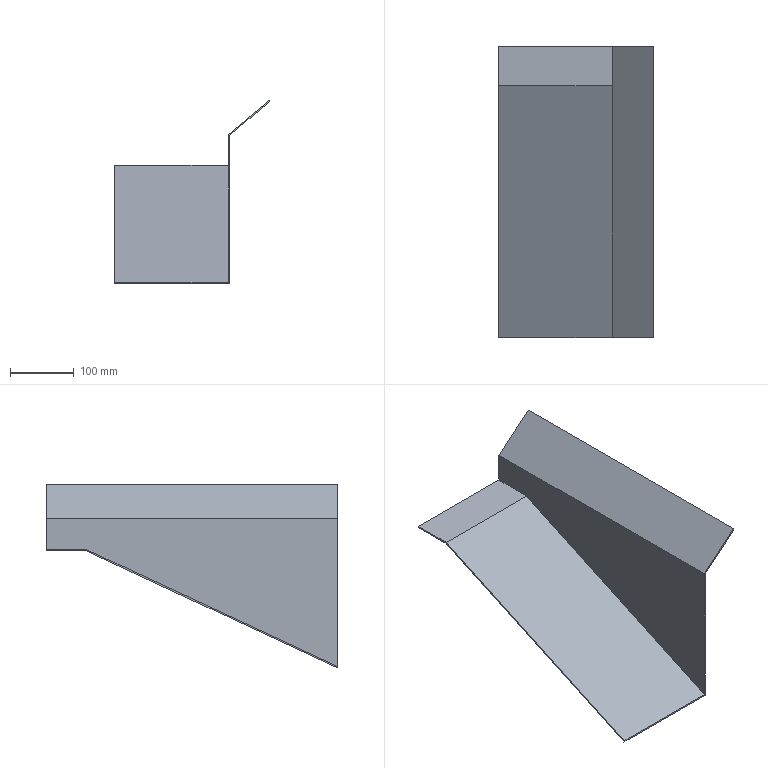Part | NX | features solid 2 | 1 solid | 12 faces | box 242.567 x 455 x 287.656 mm | volume 369224 mm3 | plane 12
STEP:
#1=CARTESIAN_POINT('',(-787.433,-30.,-47.193));
#2=VERTEX_POINT('',#1);
#3=CARTESIAN_POINT('',(-787.433,-30.,-49.804));
#4=VERTEX_POINT('',#3);
#5=CARTESIAN_POINT('',(-787.433,-30.,-303.571));
#6=DIRECTION('',(0.,0.,-1.));
#7=VECTOR('',#6,1000.);
#8=LINE('',#5,#7);
#9=EDGE_CURVE('',#2,#4,#8,.T.);
#10=ORIENTED_EDGE('',*,*,#9,.F.);
#11=CARTESIAN_POINT('',(-787.433,-485.,-47.193));
#12=VERTEX_POINT('',#11);
#13=CARTESIAN_POINT('',(-787.433,-485.,-47.193));
#14=DIRECTION('',(0.,1.,0.));
#15=VECTOR('',#14,1000.);
#16=LINE('',#13,#15);
#17=EDGE_CURVE('',#2,#12,#16,.F.);
#18=ORIENTED_EDGE('',*,*,#17,.T.);
#19=CARTESIAN_POINT('',(-787.433,-485.,-49.804));
#20=VERTEX_POINT('',#19);
#21=CARTESIAN_POINT('',(-787.433,-485.,-75.));
#22=DIRECTION('',(0.,0.,-1.));
#23=VECTOR('',#22,1000.);
#24=LINE('',#21,#23);
#25=EDGE_CURVE('',#12,#20,#24,.T.);
#26=ORIENTED_EDGE('',*,*,#25,.T.);
#27=CARTESIAN_POINT('',(-787.433,-75.,-49.804));
#28=DIRECTION('',(0.,1.,0.));
#29=VECTOR('',#28,1000.);
#30=LINE('',#27,#29);
#31=EDGE_CURVE('',#20,#4,#30,.T.);
#32=ORIENTED_EDGE('',*,*,#31,.T.);
#33=EDGE_LOOP('',(#10,#18,#26,#32));
#34=FACE_BOUND('',#33,.T.);
#35=CARTESIAN_POINT('',(-787.433,-465.,-90.));
#36=DIRECTION('',(1.,0.,0.));
#37=DIRECTION('',(0.,0.,-1.));
#38=AXIS2_PLACEMENT_3D('',#35,#36,#37);
#39=PLANE('',#38);
#40=ADVANCED_FACE('',(#34),#39,.T.);
#41=ORIENTED_EDGE('',*,*,#31,.F.);
#42=CARTESIAN_POINT('',(-850.,-485.,-102.304));
#43=VERTEX_POINT('',#42);
#44=CARTESIAN_POINT('',(-758.461,-485.,-25.493));
#45=DIRECTION('',(0.766,0.,0.6428));
#46=VECTOR('',#45,1000.);
#47=LINE('',#44,#46);
#48=EDGE_CURVE('',#43,#20,#47,.T.);
#49=ORIENTED_EDGE('',*,*,#48,.F.);
#50=CARTESIAN_POINT('',(-850.,-30.,-102.304));
#51=VERTEX_POINT('',#50);
#52=CARTESIAN_POINT('',(-850.,-75.,-102.304));
#53=DIRECTION('',(0.,1.,0.));
#54=VECTOR('',#53,1000.);
#55=LINE('',#52,#54);
#56=EDGE_CURVE('',#51,#43,#55,.F.);
#57=ORIENTED_EDGE('',*,*,#56,.F.);
#58=CARTESIAN_POINT('',(-931.5,-30.,-170.69));
#59=DIRECTION('',(0.766,0.,0.6428));
#60=VECTOR('',#59,1000.);
#61=LINE('',#58,#60);
#62=EDGE_CURVE('',#51,#4,#61,.T.);
#63=ORIENTED_EDGE('',*,*,#62,.T.);
#64=EDGE_LOOP('',(#41,#49,#57,#63));
#65=FACE_BOUND('',#64,.T.);
#66=CARTESIAN_POINT('',(-823.368,-75.,-79.957));
#67=DIRECTION('',(-0.6428,0.,0.766));
#68=DIRECTION('',(0.,-1.,0.));
#69=AXIS2_PLACEMENT_3D('',#66,#67,#68);
#70=PLANE('',#69);
#71=ADVANCED_FACE('',(#65),#70,.F.);
#72=ORIENTED_EDGE('',*,*,#17,.F.);
#73=CARTESIAN_POINT('',(-852.,-30.,-101.371));
#74=VERTEX_POINT('',#73);
#75=CARTESIAN_POINT('',(-932.786,-30.,-169.158));
#76=DIRECTION('',(0.766,0.,0.6428));
#77=VECTOR('',#76,1000.);
#78=LINE('',#75,#77);
#79=EDGE_CURVE('',#2,#74,#78,.F.);
#80=ORIENTED_EDGE('',*,*,#79,.T.);
#81=CARTESIAN_POINT('',(-852.,-485.,-101.371));
#82=VERTEX_POINT('',#81);
#83=CARTESIAN_POINT('',(-852.,-485.,-101.371));
#84=DIRECTION('',(0.,1.,0.));
#85=VECTOR('',#84,1000.);
#86=LINE('',#83,#85);
#87=EDGE_CURVE('',#74,#82,#86,.F.);
#88=ORIENTED_EDGE('',*,*,#87,.T.);
#89=CARTESIAN_POINT('',(-759.746,-485.,-23.961));
#90=DIRECTION('',(0.766,0.,0.6428));
#91=VECTOR('',#90,1000.);
#92=LINE('',#89,#91);
#93=EDGE_CURVE('',#12,#82,#92,.F.);
#94=ORIENTED_EDGE('',*,*,#93,.F.);
#95=EDGE_LOOP('',(#72,#80,#88,#94));
#96=FACE_BOUND('',#95,.T.);
#97=CARTESIAN_POINT('',(-826.288,-485.,-79.796));
#98=DIRECTION('',(-0.6428,0.,0.766));
#99=DIRECTION('',(0.766,0.,0.6428));
#100=AXIS2_PLACEMENT_3D('',#97,#98,#99);
#101=PLANE('',#100);
#102=ADVANCED_FACE('',(#96),#101,.T.);
#103=ORIENTED_EDGE('',*,*,#79,.F.);
#104=ORIENTED_EDGE('',*,*,#9,.T.);
#105=ORIENTED_EDGE('',*,*,#62,.F.);
#106=CARTESIAN_POINT('',(-850.,-30.,-151.155));
#107=VERTEX_POINT('',#106);
#108=CARTESIAN_POINT('',(-850.,-30.,-303.571));
#109=DIRECTION('',(0.,0.,-1.));
#110=VECTOR('',#109,1000.);
#111=LINE('',#108,#110);
#112=EDGE_CURVE('',#107,#51,#111,.F.);
#113=ORIENTED_EDGE('',*,*,#112,.F.);
#114=CARTESIAN_POINT('',(-1030.,-30.,-151.155));
#115=VERTEX_POINT('',#114);
#116=CARTESIAN_POINT('',(-822.,-30.,-151.155));
#117=DIRECTION('',(-1.,0.,0.));
#118=VECTOR('',#117,1000.);
#119=LINE('',#116,#118);
#120=EDGE_CURVE('',#115,#107,#119,.F.);
#121=ORIENTED_EDGE('',*,*,#120,.F.);
#122=CARTESIAN_POINT('',(-1030.,-30.,-149.155));
#123=VERTEX_POINT('',#122);
#124=CARTESIAN_POINT('',(-1030.,-30.,-303.571));
#125=DIRECTION('',(0.,0.,-1.));
#126=VECTOR('',#125,1000.);
#127=LINE('',#124,#126);
#128=EDGE_CURVE('',#123,#115,#127,.T.);
#129=ORIENTED_EDGE('',*,*,#128,.F.);
#130=CARTESIAN_POINT('',(-852.,-30.,-149.155));
#131=VERTEX_POINT('',#130);
#132=CARTESIAN_POINT('',(-822.,-30.,-149.155));
#133=DIRECTION('',(-1.,0.,0.));
#134=VECTOR('',#133,1000.);
#135=LINE('',#132,#134);
#136=EDGE_CURVE('',#123,#131,#135,.F.);
#137=ORIENTED_EDGE('',*,*,#136,.T.);
#138=CARTESIAN_POINT('',(-852.,-30.,-303.571));
#139=DIRECTION('',(0.,0.,-1.));
#140=VECTOR('',#139,1000.);
#141=LINE('',#138,#140);
#142=EDGE_CURVE('',#74,#131,#141,.T.);
#143=ORIENTED_EDGE('',*,*,#142,.F.);
#144=EDGE_LOOP('',(#103,#104,#105,#113,#121,#129,#137,#143));
#145=FACE_BOUND('',#144,.T.);
#146=CARTESIAN_POINT('',(-820.,-30.,-303.571));
#147=DIRECTION('',(0.,1.,0.));
#148=DIRECTION('',(0.,0.,1.));
#149=AXIS2_PLACEMENT_3D('',#146,#147,#148);
#150=PLANE('',#149);
#151=ADVANCED_FACE('',(#145),#150,.T.);
#152=ORIENTED_EDGE('',*,*,#25,.F.);
#153=ORIENTED_EDGE('',*,*,#93,.T.);
#154=CARTESIAN_POINT('',(-852.,-485.,-332.642));
#155=VERTEX_POINT('',#154);
#156=CARTESIAN_POINT('',(-852.,-485.,-75.));
#157=DIRECTION('',(0.,0.,-1.));
#158=VECTOR('',#157,1000.);
#159=LINE('',#156,#158);
#160=EDGE_CURVE('',#82,#155,#159,.T.);
#161=ORIENTED_EDGE('',*,*,#160,.T.);
#162=CARTESIAN_POINT('',(-1030.,-485.,-332.642));
#163=VERTEX_POINT('',#162);
#164=CARTESIAN_POINT('',(-716.919,-485.,-332.642));
#165=DIRECTION('',(1.,0.,0.));
#166=VECTOR('',#165,1000.);
#167=LINE('',#164,#166);
#168=EDGE_CURVE('',#163,#155,#167,.T.);
#169=ORIENTED_EDGE('',*,*,#168,.F.);
#170=CARTESIAN_POINT('',(-1030.,-485.,-334.848));
#171=VERTEX_POINT('',#170);
#172=CARTESIAN_POINT('',(-1030.,-485.,-75.));
#173=DIRECTION('',(0.,0.,-1.));
#174=VECTOR('',#173,1000.);
#175=LINE('',#172,#174);
#176=EDGE_CURVE('',#163,#171,#175,.T.);
#177=ORIENTED_EDGE('',*,*,#176,.T.);
#178=CARTESIAN_POINT('',(-850.,-485.,-334.848));
#179=VERTEX_POINT('',#178);
#180=CARTESIAN_POINT('',(-716.919,-485.,-334.848));
#181=DIRECTION('',(1.,0.,0.));
#182=VECTOR('',#181,1000.);
#183=LINE('',#180,#182);
#184=EDGE_CURVE('',#171,#179,#183,.T.);
#185=ORIENTED_EDGE('',*,*,#184,.T.);
#186=CARTESIAN_POINT('',(-850.,-485.,-303.571));
#187=DIRECTION('',(0.,0.,1.));
#188=VECTOR('',#187,1000.);
#189=LINE('',#186,#188);
#190=EDGE_CURVE('',#43,#179,#189,.F.);
#191=ORIENTED_EDGE('',*,*,#190,.F.);
#192=ORIENTED_EDGE('',*,*,#48,.T.);
#193=EDGE_LOOP('',(#152,#153,#161,#169,#177,#185,#191,#192));
#194=FACE_BOUND('',#193,.T.);
#195=CARTESIAN_POINT('',(-716.919,-485.,-75.));
#196=DIRECTION('',(0.,1.,0.));
#197=DIRECTION('',(0.,0.,1.));
#198=AXIS2_PLACEMENT_3D('',#195,#196,#197);
#199=PLANE('',#198);
#200=ADVANCED_FACE('',(#194),#199,.F.);
#201=CARTESIAN_POINT('',(-850.,-91.067,-151.155));
#202=VERTEX_POINT('',#201);
#203=CARTESIAN_POINT('',(-1030.,-91.067,-151.155));
#204=VERTEX_POINT('',#203);
#205=CARTESIAN_POINT('',(-822.,-91.067,-151.155));
#206=DIRECTION('',(1.,0.,0.));
#207=VECTOR('',#206,1000.);
#208=LINE('',#205,#207);
#209=EDGE_CURVE('',#202,#204,#208,.F.);
#210=ORIENTED_EDGE('',*,*,#209,.F.);
#211=CARTESIAN_POINT('',(-850.,-587.017,-382.42));
#212=DIRECTION('',(0.,-0.9063,-0.4226));
#213=VECTOR('',#212,1000.);
#214=LINE('',#211,#213);
#215=EDGE_CURVE('',#179,#202,#214,.F.);
#216=ORIENTED_EDGE('',*,*,#215,.F.);
#217=ORIENTED_EDGE('',*,*,#184,.F.);
#218=CARTESIAN_POINT('',(-1030.,-587.017,-382.42));
#219=DIRECTION('',(0.,0.9063,0.4226));
#220=VECTOR('',#219,1000.);
#221=LINE('',#218,#220);
#222=EDGE_CURVE('',#171,#204,#221,.T.);
#223=ORIENTED_EDGE('',*,*,#222,.T.);
#224=EDGE_LOOP('',(#210,#216,#217,#223));
#225=FACE_BOUND('',#224,.T.);
#226=CARTESIAN_POINT('',(-930.,-587.017,-382.42));
#227=DIRECTION('',(0.,-0.4226,0.9063));
#228=DIRECTION('',(1.,0.,0.));
#229=AXIS2_PLACEMENT_3D('',#226,#227,#228);
#230=PLANE('',#229);
#231=ADVANCED_FACE('',(#225),#230,.F.);
#232=CARTESIAN_POINT('',(-852.,-91.511,-149.155));
#233=VERTEX_POINT('',#232);
#234=CARTESIAN_POINT('',(-852.,-587.862,-380.607));
#235=DIRECTION('',(0.,0.9063,0.4226));
#236=VECTOR('',#235,1000.);
#237=LINE('',#234,#236);
#238=EDGE_CURVE('',#155,#233,#237,.T.);
#239=ORIENTED_EDGE('',*,*,#238,.T.);
#240=CARTESIAN_POINT('',(-1030.,-91.511,-149.155));
#241=VERTEX_POINT('',#240);
#242=CARTESIAN_POINT('',(-822.,-91.511,-149.155));
#243=DIRECTION('',(1.,0.,0.));
#244=VECTOR('',#243,1000.);
#245=LINE('',#242,#244);
#246=EDGE_CURVE('',#233,#241,#245,.F.);
#247=ORIENTED_EDGE('',*,*,#246,.T.);
#248=CARTESIAN_POINT('',(-1030.,-587.862,-380.607));
#249=DIRECTION('',(0.,0.9063,0.4226));
#250=VECTOR('',#249,1000.);
#251=LINE('',#248,#250);
#252=EDGE_CURVE('',#163,#241,#251,.T.);
#253=ORIENTED_EDGE('',*,*,#252,.F.);
#254=ORIENTED_EDGE('',*,*,#168,.T.);
#255=EDGE_LOOP('',(#239,#247,#253,#254));
#256=FACE_BOUND('',#255,.T.);
#257=CARTESIAN_POINT('',(-930.,-587.862,-380.607));
#258=DIRECTION('',(0.,-0.4226,0.9063));
#259=DIRECTION('',(1.,0.,0.));
#260=AXIS2_PLACEMENT_3D('',#257,#258,#259);
#261=PLANE('',#260);
#262=ADVANCED_FACE('',(#256),#261,.T.);
#263=ORIENTED_EDGE('',*,*,#252,.T.);
#264=CARTESIAN_POINT('',(-1030.,-75.,-149.155));
#265=DIRECTION('',(0.,1.,0.));
#266=VECTOR('',#265,1000.);
#267=LINE('',#264,#266);
#268=EDGE_CURVE('',#123,#241,#267,.F.);
#269=ORIENTED_EDGE('',*,*,#268,.F.);
#270=ORIENTED_EDGE('',*,*,#128,.T.);
#271=CARTESIAN_POINT('',(-1030.,-75.,-151.155));
#272=DIRECTION('',(0.,1.,0.));
#273=VECTOR('',#272,1000.);
#274=LINE('',#271,#273);
#275=EDGE_CURVE('',#115,#204,#274,.F.);
#276=ORIENTED_EDGE('',*,*,#275,.T.);
#277=ORIENTED_EDGE('',*,*,#222,.F.);
#278=ORIENTED_EDGE('',*,*,#176,.F.);
#279=EDGE_LOOP('',(#263,#269,#270,#276,#277,#278));
#280=FACE_BOUND('',#279,.T.);
#281=CARTESIAN_POINT('',(-1030.,400.,-150.));
#282=DIRECTION('',(1.,0.,0.));
#283=DIRECTION('',(0.,0.,-1.));
#284=AXIS2_PLACEMENT_3D('',#281,#282,#283);
#285=PLANE('',#284);
#286=ADVANCED_FACE('',(#280),#285,.F.);
#287=ORIENTED_EDGE('',*,*,#160,.F.);
#288=ORIENTED_EDGE('',*,*,#87,.F.);
#289=ORIENTED_EDGE('',*,*,#142,.T.);
#290=CARTESIAN_POINT('',(-852.,-75.,-149.155));
#291=DIRECTION('',(0.,1.,0.));
#292=VECTOR('',#291,1000.);
#293=LINE('',#290,#292);
#294=EDGE_CURVE('',#131,#233,#293,.F.);
#295=ORIENTED_EDGE('',*,*,#294,.T.);
#296=ORIENTED_EDGE('',*,*,#238,.F.);
#297=EDGE_LOOP('',(#287,#288,#289,#295,#296));
#298=FACE_BOUND('',#297,.T.);
#299=CARTESIAN_POINT('',(-852.,-623.785,-303.571));
#300=DIRECTION('',(1.,0.,0.));
#301=DIRECTION('',(0.,0.9063,0.4226));
#302=AXIS2_PLACEMENT_3D('',#299,#300,#301);
#303=PLANE('',#302);
#304=ADVANCED_FACE('',(#298),#303,.F.);
#305=ORIENTED_EDGE('',*,*,#56,.T.);
#306=ORIENTED_EDGE('',*,*,#190,.T.);
#307=ORIENTED_EDGE('',*,*,#215,.T.);
#308=CARTESIAN_POINT('',(-850.,-623.785,-151.155));
#309=DIRECTION('',(0.,-1.,0.));
#310=VECTOR('',#309,1000.);
#311=LINE('',#308,#310);
#312=EDGE_CURVE('',#107,#202,#311,.T.);
#313=ORIENTED_EDGE('',*,*,#312,.F.);
#314=ORIENTED_EDGE('',*,*,#112,.T.);
#315=EDGE_LOOP('',(#305,#306,#307,#313,#314));
#316=FACE_BOUND('',#315,.T.);
#317=CARTESIAN_POINT('',(-850.,-623.785,-303.571));
#318=DIRECTION('',(1.,0.,0.));
#319=DIRECTION('',(0.,0.9063,0.4226));
#320=AXIS2_PLACEMENT_3D('',#317,#318,#319);
#321=PLANE('',#320);
#322=ADVANCED_FACE('',(#316),#321,.T.);
#323=ORIENTED_EDGE('',*,*,#120,.T.);
#324=ORIENTED_EDGE('',*,*,#312,.T.);
#325=ORIENTED_EDGE('',*,*,#209,.T.);
#326=ORIENTED_EDGE('',*,*,#275,.F.);
#327=EDGE_LOOP('',(#323,#324,#325,#326));
#328=FACE_BOUND('',#327,.T.);
#329=CARTESIAN_POINT('',(-822.,-75.,-151.155));
#330=DIRECTION('',(0.,0.,1.));
#331=DIRECTION('',(0.,-1.,0.));
#332=AXIS2_PLACEMENT_3D('',#329,#330,#331);
#333=PLANE('',#332);
#334=ADVANCED_FACE('',(#328),#333,.F.);
#335=ORIENTED_EDGE('',*,*,#136,.F.);
#336=ORIENTED_EDGE('',*,*,#268,.T.);
#337=ORIENTED_EDGE('',*,*,#246,.F.);
#338=ORIENTED_EDGE('',*,*,#294,.F.);
#339=EDGE_LOOP('',(#335,#336,#337,#338));
#340=FACE_BOUND('',#339,.T.);
#341=CARTESIAN_POINT('',(-822.,-75.,-149.155));
#342=DIRECTION('',(0.,0.,1.));
#343=DIRECTION('',(0.,-1.,0.));
#344=AXIS2_PLACEMENT_3D('',#341,#342,#343);
#345=PLANE('',#344);
#346=ADVANCED_FACE('',(#340),#345,.T.);
#347=CLOSED_SHELL('',(#40,#71,#102,#151,#200,#231,#262,#286,#304,#322,#334,#346));
#348=MANIFOLD_SOLID_BREP('',#347);
#349=(LENGTH_UNIT()NAMED_UNIT(*)SI_UNIT(.MILLI.,.METRE.));
#350=UNCERTAINTY_MEASURE_WITH_UNIT(LENGTH_MEASURE(0.00001),#349,'','');
#351=(NAMED_UNIT(*)PLANE_ANGLE_UNIT()SI_UNIT($,.RADIAN.));
#352=(NAMED_UNIT(*)SI_UNIT($,.STERADIAN.)SOLID_ANGLE_UNIT());
#353=(GEOMETRIC_REPRESENTATION_CONTEXT(3)GLOBAL_UNCERTAINTY_ASSIGNED_CONTEXT((#350))GLOBAL_UNIT_ASSIGNED_CONTEXT((#349,#351,#352))REPRESENTATION_CONTEXT('',''));
#354=ADVANCED_BREP_SHAPE_REPRESENTATION('',(#348),#353);